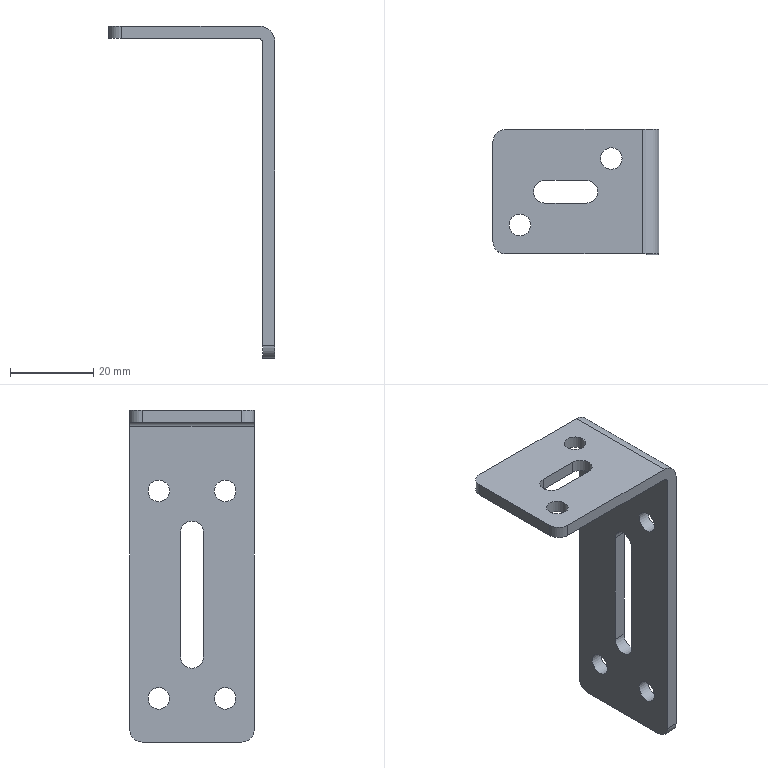Part | STEP file | YBQDJ-YB-31 | 1 solid | 28 faces | box 40 x 30 x 80 mm | volume 9225 mm3 | cylinder 16 | plane 12 | commonest cylinder face diameters 5.2 x6 5.5 x4 6 x4 2 x1 8 x1